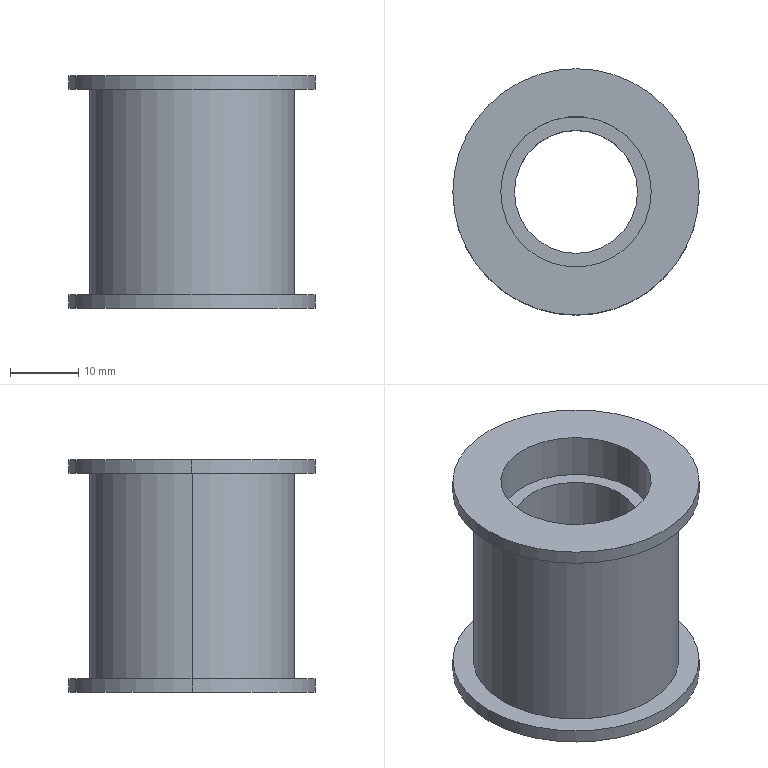Part | STEP file | (PA01.001.LX007) Tensioner Pulley | 1 solid | 18 faces | box 36 x 36 x 34 mm | volume 14967 mm3 | cylinder 12 | plane 6 | commonest cylinder face diameters 22 x4 36 x4 18 x2 30 x2
STEP:
#1=CARTESIAN_POINT('',(0.,0.,0.));
#2=DIRECTION('',(0.,0.,1.));
#3=DIRECTION('',(1.,0.,0.));
#4=AXIS2_PLACEMENT_3D('',#1,#2,#3);
#5=CARTESIAN_POINT('',(-18.,0.,-15.));
#6=VERTEX_POINT('',#5);
#7=CARTESIAN_POINT('',(18.,0.,-15.));
#8=VERTEX_POINT('',#7);
#9=CARTESIAN_POINT('',(0.,0.,-15.));
#10=DIRECTION('',(0.,0.,-1.));
#11=DIRECTION('',(-1.,0.,0.));
#12=AXIS2_PLACEMENT_3D('',#9,#10,#11);
#13=CIRCLE('',#12,18.);
#14=CARTESIAN_POINT('',(0.,0.,-15.));
#15=DIRECTION('',(0.,0.,-1.));
#16=DIRECTION('',(-1.,0.,0.));
#17=AXIS2_PLACEMENT_3D('',#14,#15,#16);
#18=CYLINDRICAL_SURFACE('',#17,18.);
#19=CARTESIAN_POINT('',(0.,0.));
#20=DIRECTION('',(1.,0.));
#21=VECTOR('',#20,1.);
#22=LINE('',#19,#21);
#23=(GEOMETRIC_REPRESENTATION_CONTEXT(2)PARAMETRIC_REPRESENTATION_CONTEXT()REPRESENTATION_CONTEXT('',''));
#24=DEFINITIONAL_REPRESENTATION('',(#22),#23);
#25=PCURVE('',#18,#24);
#26=CARTESIAN_POINT('',(0.,0.,-15.));
#27=DIRECTION('',(0.,0.,-1.));
#28=DIRECTION('',(-1.,0.,0.));
#29=AXIS2_PLACEMENT_3D('',#26,#27,#28);
#30=PLANE('',#29);
#31=CARTESIAN_POINT('',(0.,0.));
#32=DIRECTION('',(1.,0.));
#33=AXIS2_PLACEMENT_2D('',#31,#32);
#34=CIRCLE('',#33,18.);
#35=(GEOMETRIC_REPRESENTATION_CONTEXT(2)PARAMETRIC_REPRESENTATION_CONTEXT()REPRESENTATION_CONTEXT('',''));
#36=DEFINITIONAL_REPRESENTATION('',(#34),#35);
#37=PCURVE('',#30,#36);
#38=SURFACE_CURVE('',#13,(#25,#37),.PCURVE_S1.);
#39=EDGE_CURVE('',#6,#8,#38,.T.);
#40=ORIENTED_EDGE('',*,*,#39,.T.);
#41=CARTESIAN_POINT('',(18.,0.,-17.));
#42=VERTEX_POINT('',#41);
#43=CARTESIAN_POINT('',(18.,0.,-15.));
#44=DIRECTION('',(0.,0.,-1.));
#45=VECTOR('',#44,1.);
#46=LINE('',#43,#45);
#47=CARTESIAN_POINT('',(3.142,0.));
#48=DIRECTION('',(0.,1.));
#49=VECTOR('',#48,1.);
#50=LINE('',#47,#49);
#51=(GEOMETRIC_REPRESENTATION_CONTEXT(2)PARAMETRIC_REPRESENTATION_CONTEXT()REPRESENTATION_CONTEXT('',''));
#52=DEFINITIONAL_REPRESENTATION('',(#50),#51);
#53=PCURVE('',#18,#52);
#54=CARTESIAN_POINT('',(0.,0.,-15.));
#55=DIRECTION('',(0.,0.,-1.));
#56=DIRECTION('',(-1.,0.,0.));
#57=AXIS2_PLACEMENT_3D('',#54,#55,#56);
#58=CYLINDRICAL_SURFACE('',#57,18.);
#59=CARTESIAN_POINT('',(3.142,0.));
#60=DIRECTION('',(0.,1.));
#61=VECTOR('',#60,1.);
#62=LINE('',#59,#61);
#63=(GEOMETRIC_REPRESENTATION_CONTEXT(2)PARAMETRIC_REPRESENTATION_CONTEXT()REPRESENTATION_CONTEXT('',''));
#64=DEFINITIONAL_REPRESENTATION('',(#62),#63);
#65=PCURVE('',#58,#64);
#66=SURFACE_CURVE('',#46,(#53,#65),.PCURVE_S1.);
#67=EDGE_CURVE('',#8,#42,#66,.T.);
#68=ORIENTED_EDGE('',*,*,#67,.T.);
#69=CARTESIAN_POINT('',(-18.,0.,-17.));
#70=VERTEX_POINT('',#69);
#71=CARTESIAN_POINT('',(0.,0.,-17.));
#72=DIRECTION('',(0.,0.,-1.));
#73=DIRECTION('',(-1.,0.,0.));
#74=AXIS2_PLACEMENT_3D('',#71,#72,#73);
#75=CIRCLE('',#74,18.);
#76=CARTESIAN_POINT('',(0.,2.));
#77=DIRECTION('',(1.,0.));
#78=VECTOR('',#77,1.);
#79=LINE('',#76,#78);
#80=(GEOMETRIC_REPRESENTATION_CONTEXT(2)PARAMETRIC_REPRESENTATION_CONTEXT()REPRESENTATION_CONTEXT('',''));
#81=DEFINITIONAL_REPRESENTATION('',(#79),#80);
#82=PCURVE('',#18,#81);
#83=CARTESIAN_POINT('',(0.,0.,-17.));
#84=DIRECTION('',(0.,0.,1.));
#85=DIRECTION('',(1.,0.,0.));
#86=AXIS2_PLACEMENT_3D('',#83,#84,#85);
#87=PLANE('',#86);
#88=CARTESIAN_POINT('',(-18.,0.));
#89=CARTESIAN_POINT('',(-18.,31.177));
#90=CARTESIAN_POINT('',(9.,15.588));
#91=CARTESIAN_POINT('',(36.,0.));
#92=CARTESIAN_POINT('',(9.,-15.588));
#93=CARTESIAN_POINT('',(-18.,-31.177));
#94=CARTESIAN_POINT('',(-18.,0.));
#95=(BOUNDED_CURVE()B_SPLINE_CURVE(2,(#88,#89,#90,#91,#92,#93,#94),.UNSPECIFIED.,.T.,.F.)B_SPLINE_CURVE_WITH_KNOTS((1,2,2,2,2,1),(-2.094,0.,2.094,4.189,6.283,8.378),.UNSPECIFIED.)CURVE()GEOMETRIC_REPRESENTATION_ITEM()RATIONAL_B_SPLINE_CURVE((1.,0.5,1.,0.5,1.,0.5,1.))REPRESENTATION_ITEM(''));
#96=(GEOMETRIC_REPRESENTATION_CONTEXT(2)PARAMETRIC_REPRESENTATION_CONTEXT()REPRESENTATION_CONTEXT('',''));
#97=DEFINITIONAL_REPRESENTATION('',(#95),#96);
#98=PCURVE('',#87,#97);
#99=SURFACE_CURVE('',#75,(#82,#98),.PCURVE_S1.);
#100=EDGE_CURVE('',#70,#42,#99,.T.);
#101=ORIENTED_EDGE('',*,*,#100,.F.);
#102=CARTESIAN_POINT('',(-18.,0.,-15.));
#103=DIRECTION('',(0.,0.,-1.));
#104=VECTOR('',#103,1.);
#105=LINE('',#102,#104);
#106=CARTESIAN_POINT('',(0.,0.));
#107=DIRECTION('',(0.,1.));
#108=VECTOR('',#107,1.);
#109=LINE('',#106,#108);
#110=(GEOMETRIC_REPRESENTATION_CONTEXT(2)PARAMETRIC_REPRESENTATION_CONTEXT()REPRESENTATION_CONTEXT('',''));
#111=DEFINITIONAL_REPRESENTATION('',(#109),#110);
#112=PCURVE('',#18,#111);
#113=CARTESIAN_POINT('',(6.283,0.));
#114=DIRECTION('',(0.,1.));
#115=VECTOR('',#114,1.);
#116=LINE('',#113,#115);
#117=(GEOMETRIC_REPRESENTATION_CONTEXT(2)PARAMETRIC_REPRESENTATION_CONTEXT()REPRESENTATION_CONTEXT('',''));
#118=DEFINITIONAL_REPRESENTATION('',(#116),#117);
#119=PCURVE('',#58,#118);
#120=SURFACE_CURVE('',#105,(#112,#119),.PCURVE_S1.);
#121=EDGE_CURVE('',#6,#70,#120,.T.);
#122=ORIENTED_EDGE('',*,*,#121,.F.);
#123=EDGE_LOOP('',(#40,#68,#101,#122));
#124=FACE_BOUND('',#123,.T.);
#125=ADVANCED_FACE('',(#124),#18,.T.);
#126=CARTESIAN_POINT('',(18.,0.,15.));
#127=VERTEX_POINT('',#126);
#128=CARTESIAN_POINT('',(-18.,0.,15.));
#129=VERTEX_POINT('',#128);
#130=CARTESIAN_POINT('',(0.,0.,15.));
#131=DIRECTION('',(0.,0.,1.));
#132=DIRECTION('',(1.,0.,0.));
#133=AXIS2_PLACEMENT_3D('',#130,#131,#132);
#134=CIRCLE('',#133,18.);
#135=CARTESIAN_POINT('',(0.,0.,15.));
#136=DIRECTION('',(0.,0.,1.));
#137=DIRECTION('',(1.,0.,0.));
#138=AXIS2_PLACEMENT_3D('',#135,#136,#137);
#139=CYLINDRICAL_SURFACE('',#138,18.);
#140=CARTESIAN_POINT('',(0.,0.));
#141=DIRECTION('',(1.,0.));
#142=VECTOR('',#141,1.);
#143=LINE('',#140,#142);
#144=(GEOMETRIC_REPRESENTATION_CONTEXT(2)PARAMETRIC_REPRESENTATION_CONTEXT()REPRESENTATION_CONTEXT('',''));
#145=DEFINITIONAL_REPRESENTATION('',(#143),#144);
#146=PCURVE('',#139,#145);
#147=CARTESIAN_POINT('',(0.,0.,15.));
#148=DIRECTION('',(0.,0.,1.));
#149=DIRECTION('',(1.,0.,0.));
#150=AXIS2_PLACEMENT_3D('',#147,#148,#149);
#151=PLANE('',#150);
#152=CARTESIAN_POINT('',(0.,0.));
#153=DIRECTION('',(1.,0.));
#154=AXIS2_PLACEMENT_2D('',#152,#153);
#155=CIRCLE('',#154,18.);
#156=(GEOMETRIC_REPRESENTATION_CONTEXT(2)PARAMETRIC_REPRESENTATION_CONTEXT()REPRESENTATION_CONTEXT('',''));
#157=DEFINITIONAL_REPRESENTATION('',(#155),#156);
#158=PCURVE('',#151,#157);
#159=SURFACE_CURVE('',#134,(#146,#158),.PCURVE_S1.);
#160=EDGE_CURVE('',#127,#129,#159,.T.);
#161=ORIENTED_EDGE('',*,*,#160,.T.);
#162=CARTESIAN_POINT('',(-18.,0.,17.));
#163=VERTEX_POINT('',#162);
#164=CARTESIAN_POINT('',(-18.,0.,15.));
#165=DIRECTION('',(0.,0.,1.));
#166=VECTOR('',#165,1.);
#167=LINE('',#164,#166);
#168=CARTESIAN_POINT('',(3.142,0.));
#169=DIRECTION('',(0.,1.));
#170=VECTOR('',#169,1.);
#171=LINE('',#168,#170);
#172=(GEOMETRIC_REPRESENTATION_CONTEXT(2)PARAMETRIC_REPRESENTATION_CONTEXT()REPRESENTATION_CONTEXT('',''));
#173=DEFINITIONAL_REPRESENTATION('',(#171),#172);
#174=PCURVE('',#139,#173);
#175=CARTESIAN_POINT('',(0.,0.,15.));
#176=DIRECTION('',(0.,0.,1.));
#177=DIRECTION('',(1.,0.,0.));
#178=AXIS2_PLACEMENT_3D('',#175,#176,#177);
#179=CYLINDRICAL_SURFACE('',#178,18.);
#180=CARTESIAN_POINT('',(3.142,0.));
#181=DIRECTION('',(0.,1.));
#182=VECTOR('',#181,1.);
#183=LINE('',#180,#182);
#184=(GEOMETRIC_REPRESENTATION_CONTEXT(2)PARAMETRIC_REPRESENTATION_CONTEXT()REPRESENTATION_CONTEXT('',''));
#185=DEFINITIONAL_REPRESENTATION('',(#183),#184);
#186=PCURVE('',#179,#185);
#187=SURFACE_CURVE('',#167,(#174,#186),.PCURVE_S1.);
#188=EDGE_CURVE('',#129,#163,#187,.T.);
#189=ORIENTED_EDGE('',*,*,#188,.T.);
#190=CARTESIAN_POINT('',(18.,0.,17.));
#191=VERTEX_POINT('',#190);
#192=CARTESIAN_POINT('',(0.,0.,17.));
#193=DIRECTION('',(0.,0.,1.));
#194=DIRECTION('',(1.,0.,0.));
#195=AXIS2_PLACEMENT_3D('',#192,#193,#194);
#196=CIRCLE('',#195,18.);
#197=CARTESIAN_POINT('',(0.,2.));
#198=DIRECTION('',(1.,0.));
#199=VECTOR('',#198,1.);
#200=LINE('',#197,#199);
#201=(GEOMETRIC_REPRESENTATION_CONTEXT(2)PARAMETRIC_REPRESENTATION_CONTEXT()REPRESENTATION_CONTEXT('',''));
#202=DEFINITIONAL_REPRESENTATION('',(#200),#201);
#203=PCURVE('',#139,#202);
#204=CARTESIAN_POINT('',(0.,0.,17.));
#205=DIRECTION('',(0.,0.,1.));
#206=DIRECTION('',(1.,0.,0.));
#207=AXIS2_PLACEMENT_3D('',#204,#205,#206);
#208=PLANE('',#207);
#209=CARTESIAN_POINT('',(0.,0.));
#210=DIRECTION('',(1.,0.));
#211=AXIS2_PLACEMENT_2D('',#209,#210);
#212=CIRCLE('',#211,18.);
#213=(GEOMETRIC_REPRESENTATION_CONTEXT(2)PARAMETRIC_REPRESENTATION_CONTEXT()REPRESENTATION_CONTEXT('',''));
#214=DEFINITIONAL_REPRESENTATION('',(#212),#213);
#215=PCURVE('',#208,#214);
#216=SURFACE_CURVE('',#196,(#203,#215),.PCURVE_S1.);
#217=EDGE_CURVE('',#191,#163,#216,.T.);
#218=ORIENTED_EDGE('',*,*,#217,.F.);
#219=CARTESIAN_POINT('',(18.,0.,15.));
#220=DIRECTION('',(0.,0.,1.));
#221=VECTOR('',#220,1.);
#222=LINE('',#219,#221);
#223=CARTESIAN_POINT('',(0.,0.));
#224=DIRECTION('',(0.,1.));
#225=VECTOR('',#224,1.);
#226=LINE('',#223,#225);
#227=(GEOMETRIC_REPRESENTATION_CONTEXT(2)PARAMETRIC_REPRESENTATION_CONTEXT()REPRESENTATION_CONTEXT('',''));
#228=DEFINITIONAL_REPRESENTATION('',(#226),#227);
#229=PCURVE('',#139,#228);
#230=CARTESIAN_POINT('',(6.283,0.));
#231=DIRECTION('',(0.,1.));
#232=VECTOR('',#231,1.);
#233=LINE('',#230,#232);
#234=(GEOMETRIC_REPRESENTATION_CONTEXT(2)PARAMETRIC_REPRESENTATION_CONTEXT()REPRESENTATION_CONTEXT('',''));
#235=DEFINITIONAL_REPRESENTATION('',(#233),#234);
#236=PCURVE('',#179,#235);
#237=SURFACE_CURVE('',#222,(#229,#236),.PCURVE_S1.);
#238=EDGE_CURVE('',#127,#191,#237,.T.);
#239=ORIENTED_EDGE('',*,*,#238,.F.);
#240=EDGE_LOOP('',(#161,#189,#218,#239));
#241=FACE_BOUND('',#240,.T.);
#242=ADVANCED_FACE('',(#241),#139,.T.);
#243=CARTESIAN_POINT('',(9.,0.,-10.4));
#244=VERTEX_POINT('',#243);
#245=CARTESIAN_POINT('',(9.,0.,10.4));
#246=VERTEX_POINT('',#245);
#247=CARTESIAN_POINT('',(9.,0.,-17.));
#248=DIRECTION('',(0.,0.,1.));
#249=VECTOR('',#248,1.);
#250=LINE('',#247,#249);
#251=CARTESIAN_POINT('',(0.,0.,-17.));
#252=DIRECTION('',(0.,0.,1.));
#253=DIRECTION('',(1.,0.,0.));
#254=AXIS2_PLACEMENT_3D('',#251,#252,#253);
#255=CYLINDRICAL_SURFACE('',#254,9.);
#256=CARTESIAN_POINT('',(6.283,0.));
#257=DIRECTION('',(0.,1.));
#258=VECTOR('',#257,1.);
#259=LINE('',#256,#258);
#260=(GEOMETRIC_REPRESENTATION_CONTEXT(2)PARAMETRIC_REPRESENTATION_CONTEXT()REPRESENTATION_CONTEXT('',''));
#261=DEFINITIONAL_REPRESENTATION('',(#259),#260);
#262=PCURVE('',#255,#261);
#263=CARTESIAN_POINT('',(0.,0.,-17.));
#264=DIRECTION('',(0.,0.,1.));
#265=DIRECTION('',(1.,0.,0.));
#266=AXIS2_PLACEMENT_3D('',#263,#264,#265);
#267=CYLINDRICAL_SURFACE('',#266,9.);
#268=CARTESIAN_POINT('',(0.,0.));
#269=DIRECTION('',(0.,1.));
#270=VECTOR('',#269,1.);
#271=LINE('',#268,#270);
#272=(GEOMETRIC_REPRESENTATION_CONTEXT(2)PARAMETRIC_REPRESENTATION_CONTEXT()REPRESENTATION_CONTEXT('',''));
#273=DEFINITIONAL_REPRESENTATION('',(#271),#272);
#274=PCURVE('',#267,#273);
#275=SURFACE_CURVE('',#250,(#262,#274),.PCURVE_S1.);
#276=EDGE_CURVE('',#244,#246,#275,.T.);
#277=ORIENTED_EDGE('',*,*,#276,.T.);
#278=CARTESIAN_POINT('',(-9.,0.,10.4));
#279=VERTEX_POINT('',#278);
#280=CARTESIAN_POINT('',(0.,0.,10.4));
#281=DIRECTION('',(0.,0.,1.));
#282=DIRECTION('',(1.,0.,0.));
#283=AXIS2_PLACEMENT_3D('',#280,#281,#282);
#284=CIRCLE('',#283,9.);
#285=CARTESIAN_POINT('',(0.,27.4));
#286=DIRECTION('',(1.,0.));
#287=VECTOR('',#286,1.);
#288=LINE('',#285,#287);
#289=(GEOMETRIC_REPRESENTATION_CONTEXT(2)PARAMETRIC_REPRESENTATION_CONTEXT()REPRESENTATION_CONTEXT('',''));
#290=DEFINITIONAL_REPRESENTATION('',(#288),#289);
#291=PCURVE('',#255,#290);
#292=CARTESIAN_POINT('',(0.,0.,10.4));
#293=DIRECTION('',(0.,0.,1.));
#294=DIRECTION('',(1.,0.,0.));
#295=AXIS2_PLACEMENT_3D('',#292,#293,#294);
#296=PLANE('',#295);
#297=CARTESIAN_POINT('',(0.,0.));
#298=DIRECTION('',(1.,0.));
#299=AXIS2_PLACEMENT_2D('',#297,#298);
#300=CIRCLE('',#299,9.);
#301=(GEOMETRIC_REPRESENTATION_CONTEXT(2)PARAMETRIC_REPRESENTATION_CONTEXT()REPRESENTATION_CONTEXT('',''));
#302=DEFINITIONAL_REPRESENTATION('',(#300),#301);
#303=PCURVE('',#296,#302);
#304=SURFACE_CURVE('',#284,(#291,#303),.PCURVE_S1.);
#305=EDGE_CURVE('',#279,#246,#304,.T.);
#306=ORIENTED_EDGE('',*,*,#305,.F.);
#307=CARTESIAN_POINT('',(-9.,0.,-10.4));
#308=VERTEX_POINT('',#307);
#309=CARTESIAN_POINT('',(-9.,0.,-17.));
#310=DIRECTION('',(0.,0.,1.));
#311=VECTOR('',#310,1.);
#312=LINE('',#309,#311);
#313=CARTESIAN_POINT('',(3.142,0.));
#314=DIRECTION('',(0.,1.));
#315=VECTOR('',#314,1.);
#316=LINE('',#313,#315);
#317=(GEOMETRIC_REPRESENTATION_CONTEXT(2)PARAMETRIC_REPRESENTATION_CONTEXT()REPRESENTATION_CONTEXT('',''));
#318=DEFINITIONAL_REPRESENTATION('',(#316),#317);
#319=PCURVE('',#255,#318);
#320=CARTESIAN_POINT('',(3.142,0.));
#321=DIRECTION('',(0.,1.));
#322=VECTOR('',#321,1.);
#323=LINE('',#320,#322);
#324=(GEOMETRIC_REPRESENTATION_CONTEXT(2)PARAMETRIC_REPRESENTATION_CONTEXT()REPRESENTATION_CONTEXT('',''));
#325=DEFINITIONAL_REPRESENTATION('',(#323),#324);
#326=PCURVE('',#267,#325);
#327=SURFACE_CURVE('',#312,(#319,#326),.PCURVE_S1.);
#328=EDGE_CURVE('',#308,#279,#327,.T.);
#329=ORIENTED_EDGE('',*,*,#328,.F.);
#330=CARTESIAN_POINT('',(0.,0.,-10.4));
#331=DIRECTION('',(0.,0.,-1.));
#332=DIRECTION('',(-1.,0.,0.));
#333=AXIS2_PLACEMENT_3D('',#330,#331,#332);
#334=CIRCLE('',#333,9.);
#335=CARTESIAN_POINT('',(9.425,6.6));
#336=DIRECTION('',(-1.,0.));
#337=VECTOR('',#336,1.);
#338=LINE('',#335,#337);
#339=(GEOMETRIC_REPRESENTATION_CONTEXT(2)PARAMETRIC_REPRESENTATION_CONTEXT()REPRESENTATION_CONTEXT('',''));
#340=DEFINITIONAL_REPRESENTATION('',(#338),#339);
#341=PCURVE('',#255,#340);
#342=CARTESIAN_POINT('',(0.,0.,-10.4));
#343=DIRECTION('',(0.,0.,-1.));
#344=DIRECTION('',(1.,0.,0.));
#345=AXIS2_PLACEMENT_3D('',#342,#343,#344);
#346=PLANE('',#345);
#347=CARTESIAN_POINT('',(0.,0.));
#348=DIRECTION('',(-1.,0.));
#349=AXIS2_PLACEMENT_2D('',#347,#348);
#350=CIRCLE('',#349,9.);
#351=(GEOMETRIC_REPRESENTATION_CONTEXT(2)PARAMETRIC_REPRESENTATION_CONTEXT()REPRESENTATION_CONTEXT('',''));
#352=DEFINITIONAL_REPRESENTATION('',(#350),#351);
#353=PCURVE('',#346,#352);
#354=SURFACE_CURVE('',#334,(#341,#353),.PCURVE_S1.);
#355=EDGE_CURVE('',#244,#308,#354,.T.);
#356=ORIENTED_EDGE('',*,*,#355,.F.);
#357=EDGE_LOOP('',(#277,#306,#329,#356));
#358=FACE_BOUND('',#357,.F.);
#359=ADVANCED_FACE('',(#358),#255,.F.);
#360=CARTESIAN_POINT('',(-11.,0.,-10.4));
#361=VERTEX_POINT('',#360);
#362=CARTESIAN_POINT('',(-11.,0.,-17.));
#363=VERTEX_POINT('',#362);
#364=CARTESIAN_POINT('',(-11.,0.,-10.4));
#365=DIRECTION('',(0.,0.,-1.));
#366=VECTOR('',#365,1.);
#367=LINE('',#364,#366);
#368=CARTESIAN_POINT('',(0.,0.,-10.4));
#369=DIRECTION('',(0.,0.,-1.));
#370=DIRECTION('',(-1.,0.,0.));
#371=AXIS2_PLACEMENT_3D('',#368,#369,#370);
#372=CYLINDRICAL_SURFACE('',#371,11.);
#373=CARTESIAN_POINT('',(6.283,0.));
#374=DIRECTION('',(0.,1.));
#375=VECTOR('',#374,1.);
#376=LINE('',#373,#375);
#377=(GEOMETRIC_REPRESENTATION_CONTEXT(2)PARAMETRIC_REPRESENTATION_CONTEXT()REPRESENTATION_CONTEXT('',''));
#378=DEFINITIONAL_REPRESENTATION('',(#376),#377);
#379=PCURVE('',#372,#378);
#380=CARTESIAN_POINT('',(0.,0.,-10.4));
#381=DIRECTION('',(0.,0.,-1.));
#382=DIRECTION('',(-1.,0.,0.));
#383=AXIS2_PLACEMENT_3D('',#380,#381,#382);
#384=CYLINDRICAL_SURFACE('',#383,11.);
#385=CARTESIAN_POINT('',(0.,0.));
#386=DIRECTION('',(0.,1.));
#387=VECTOR('',#386,1.);
#388=LINE('',#385,#387);
#389=(GEOMETRIC_REPRESENTATION_CONTEXT(2)PARAMETRIC_REPRESENTATION_CONTEXT()REPRESENTATION_CONTEXT('',''));
#390=DEFINITIONAL_REPRESENTATION('',(#388),#389);
#391=PCURVE('',#384,#390);
#392=SURFACE_CURVE('',#367,(#379,#391),.PCURVE_S1.);
#393=EDGE_CURVE('',#361,#363,#392,.T.);
#394=ORIENTED_EDGE('',*,*,#393,.T.);
#395=CARTESIAN_POINT('',(11.,0.,-17.));
#396=VERTEX_POINT('',#395);
#397=CARTESIAN_POINT('',(0.,0.,-17.));
#398=DIRECTION('',(0.,0.,1.));
#399=DIRECTION('',(1.,0.,0.));
#400=AXIS2_PLACEMENT_3D('',#397,#398,#399);
#401=CIRCLE('',#400,11.);
#402=CARTESIAN_POINT('',(9.425,6.6));
#403=DIRECTION('',(-1.,0.));
#404=VECTOR('',#403,1.);
#405=LINE('',#402,#404);
#406=(GEOMETRIC_REPRESENTATION_CONTEXT(2)PARAMETRIC_REPRESENTATION_CONTEXT()REPRESENTATION_CONTEXT('',''));
#407=DEFINITIONAL_REPRESENTATION('',(#405),#406);
#408=PCURVE('',#372,#407);
#409=CARTESIAN_POINT('',(0.,0.));
#410=DIRECTION('',(1.,0.));
#411=AXIS2_PLACEMENT_2D('',#409,#410);
#412=CIRCLE('',#411,11.);
#413=(GEOMETRIC_REPRESENTATION_CONTEXT(2)PARAMETRIC_REPRESENTATION_CONTEXT()REPRESENTATION_CONTEXT('',''));
#414=DEFINITIONAL_REPRESENTATION('',(#412),#413);
#415=PCURVE('',#87,#414);
#416=SURFACE_CURVE('',#401,(#408,#415),.PCURVE_S1.);
#417=EDGE_CURVE('',#363,#396,#416,.T.);
#418=ORIENTED_EDGE('',*,*,#417,.T.);
#419=CARTESIAN_POINT('',(11.,0.,-10.4));
#420=VERTEX_POINT('',#419);
#421=CARTESIAN_POINT('',(11.,0.,-10.4));
#422=DIRECTION('',(0.,0.,-1.));
#423=VECTOR('',#422,1.);
#424=LINE('',#421,#423);
#425=CARTESIAN_POINT('',(3.142,0.));
#426=DIRECTION('',(0.,1.));
#427=VECTOR('',#426,1.);
#428=LINE('',#425,#427);
#429=(GEOMETRIC_REPRESENTATION_CONTEXT(2)PARAMETRIC_REPRESENTATION_CONTEXT()REPRESENTATION_CONTEXT('',''));
#430=DEFINITIONAL_REPRESENTATION('',(#428),#429);
#431=PCURVE('',#372,#430);
#432=CARTESIAN_POINT('',(3.142,0.));
#433=DIRECTION('',(0.,1.));
#434=VECTOR('',#433,1.);
#435=LINE('',#432,#434);
#436=(GEOMETRIC_REPRESENTATION_CONTEXT(2)PARAMETRIC_REPRESENTATION_CONTEXT()REPRESENTATION_CONTEXT('',''));
#437=DEFINITIONAL_REPRESENTATION('',(#435),#436);
#438=PCURVE('',#384,#437);
#439=SURFACE_CURVE('',#424,(#431,#438),.PCURVE_S1.);
#440=EDGE_CURVE('',#420,#396,#439,.T.);
#441=ORIENTED_EDGE('',*,*,#440,.F.);
#442=CARTESIAN_POINT('',(0.,0.,-10.4));
#443=DIRECTION('',(0.,0.,1.));
#444=DIRECTION('',(1.,0.,0.));
#445=AXIS2_PLACEMENT_3D('',#442,#443,#444);
#446=CIRCLE('',#445,11.);
#447=CARTESIAN_POINT('',(9.425,0.));
#448=DIRECTION('',(-1.,0.));
#449=VECTOR('',#448,1.);
#450=LINE('',#447,#449);
#451=(GEOMETRIC_REPRESENTATION_CONTEXT(2)PARAMETRIC_REPRESENTATION_CONTEXT()REPRESENTATION_CONTEXT('',''));
#452=DEFINITIONAL_REPRESENTATION('',(#450),#451);
#453=PCURVE('',#372,#452);
#454=CARTESIAN_POINT('',(11.,0.));
#455=CARTESIAN_POINT('',(11.,-19.053));
#456=CARTESIAN_POINT('',(-5.5,-9.526));
#457=CARTESIAN_POINT('',(-22.,0.));
#458=CARTESIAN_POINT('',(-5.5,9.526));
#459=CARTESIAN_POINT('',(11.,19.053));
#460=CARTESIAN_POINT('',(11.,0.));
#461=(BOUNDED_CURVE()B_SPLINE_CURVE(2,(#454,#455,#456,#457,#458,#459,#460),.UNSPECIFIED.,.T.,.F.)B_SPLINE_CURVE_WITH_KNOTS((1,2,2,2,2,1),(-2.094,0.,2.094,4.189,6.283,8.378),.UNSPECIFIED.)CURVE()GEOMETRIC_REPRESENTATION_ITEM()RATIONAL_B_SPLINE_CURVE((1.,0.5,1.,0.5,1.,0.5,1.))REPRESENTATION_ITEM(''));
#462=(GEOMETRIC_REPRESENTATION_CONTEXT(2)PARAMETRIC_REPRESENTATION_CONTEXT()REPRESENTATION_CONTEXT('',''));
#463=DEFINITIONAL_REPRESENTATION('',(#461),#462);
#464=PCURVE('',#346,#463);
#465=SURFACE_CURVE('',#446,(#453,#464),.PCURVE_S1.);
#466=EDGE_CURVE('',#361,#420,#465,.T.);
#467=ORIENTED_EDGE('',*,*,#466,.F.);
#468=EDGE_LOOP('',(#394,#418,#441,#467));
#469=FACE_BOUND('',#468,.F.);
#470=ADVANCED_FACE('',(#469),#372,.F.);
#471=CARTESIAN_POINT('',(11.,0.,10.4));
#472=VERTEX_POINT('',#471);
#473=CARTESIAN_POINT('',(11.,0.,17.));
#474=VERTEX_POINT('',#473);
#475=CARTESIAN_POINT('',(11.,0.,10.4));
#476=DIRECTION('',(0.,0.,1.));
#477=VECTOR('',#476,1.);
#478=LINE('',#475,#477);
#479=CARTESIAN_POINT('',(0.,0.,10.4));
#480=DIRECTION('',(0.,0.,1.));
#481=DIRECTION('',(1.,0.,0.));
#482=AXIS2_PLACEMENT_3D('',#479,#480,#481);
#483=CYLINDRICAL_SURFACE('',#482,11.);
#484=CARTESIAN_POINT('',(6.283,0.));
#485=DIRECTION('',(0.,1.));
#486=VECTOR('',#485,1.);
#487=LINE('',#484,#486);
#488=(GEOMETRIC_REPRESENTATION_CONTEXT(2)PARAMETRIC_REPRESENTATION_CONTEXT()REPRESENTATION_CONTEXT('',''));
#489=DEFINITIONAL_REPRESENTATION('',(#487),#488);
#490=PCURVE('',#483,#489);
#491=CARTESIAN_POINT('',(0.,0.,10.4));
#492=DIRECTION('',(0.,0.,1.));
#493=DIRECTION('',(1.,0.,0.));
#494=AXIS2_PLACEMENT_3D('',#491,#492,#493);
#495=CYLINDRICAL_SURFACE('',#494,11.);
#496=CARTESIAN_POINT('',(0.,0.));
#497=DIRECTION('',(0.,1.));
#498=VECTOR('',#497,1.);
#499=LINE('',#496,#498);
#500=(GEOMETRIC_REPRESENTATION_CONTEXT(2)PARAMETRIC_REPRESENTATION_CONTEXT()REPRESENTATION_CONTEXT('',''));
#501=DEFINITIONAL_REPRESENTATION('',(#499),#500);
#502=PCURVE('',#495,#501);
#503=SURFACE_CURVE('',#478,(#490,#502),.PCURVE_S1.);
#504=EDGE_CURVE('',#472,#474,#503,.T.);
#505=ORIENTED_EDGE('',*,*,#504,.T.);
#506=CARTESIAN_POINT('',(-11.,0.,17.));
#507=VERTEX_POINT('',#506);
#508=CARTESIAN_POINT('',(0.,0.,17.));
#509=DIRECTION('',(0.,0.,1.));
#510=DIRECTION('',(1.,0.,0.));
#511=AXIS2_PLACEMENT_3D('',#508,#509,#510);
#512=CIRCLE('',#511,11.);
#513=CARTESIAN_POINT('',(0.,6.6));
#514=DIRECTION('',(1.,0.));
#515=VECTOR('',#514,1.);
#516=LINE('',#513,#515);
#517=(GEOMETRIC_REPRESENTATION_CONTEXT(2)PARAMETRIC_REPRESENTATION_CONTEXT()REPRESENTATION_CONTEXT('',''));
#518=DEFINITIONAL_REPRESENTATION('',(#516),#517);
#519=PCURVE('',#483,#518);
#520=CARTESIAN_POINT('',(0.,0.));
#521=DIRECTION('',(1.,0.));
#522=AXIS2_PLACEMENT_2D('',#520,#521);
#523=CIRCLE('',#522,11.);
#524=(GEOMETRIC_REPRESENTATION_CONTEXT(2)PARAMETRIC_REPRESENTATION_CONTEXT()REPRESENTATION_CONTEXT('',''));
#525=DEFINITIONAL_REPRESENTATION('',(#523),#524);
#526=PCURVE('',#208,#525);
#527=SURFACE_CURVE('',#512,(#519,#526),.PCURVE_S1.);
#528=EDGE_CURVE('',#507,#474,#527,.T.);
#529=ORIENTED_EDGE('',*,*,#528,.F.);
#530=CARTESIAN_POINT('',(-11.,0.,10.4));
#531=VERTEX_POINT('',#530);
#532=CARTESIAN_POINT('',(-11.,0.,10.4));
#533=DIRECTION('',(0.,0.,1.));
#534=VECTOR('',#533,1.);
#535=LINE('',#532,#534);
#536=CARTESIAN_POINT('',(3.142,0.));
#537=DIRECTION('',(0.,1.));
#538=VECTOR('',#537,1.);
#539=LINE('',#536,#538);
#540=(GEOMETRIC_REPRESENTATION_CONTEXT(2)PARAMETRIC_REPRESENTATION_CONTEXT()REPRESENTATION_CONTEXT('',''));
#541=DEFINITIONAL_REPRESENTATION('',(#539),#540);
#542=PCURVE('',#483,#541);
#543=CARTESIAN_POINT('',(3.142,0.));
#544=DIRECTION('',(0.,1.));
#545=VECTOR('',#544,1.);
#546=LINE('',#543,#545);
#547=(GEOMETRIC_REPRESENTATION_CONTEXT(2)PARAMETRIC_REPRESENTATION_CONTEXT()REPRESENTATION_CONTEXT('',''));
#548=DEFINITIONAL_REPRESENTATION('',(#546),#547);
#549=PCURVE('',#495,#548);
#550=SURFACE_CURVE('',#535,(#542,#549),.PCURVE_S1.);
#551=EDGE_CURVE('',#531,#507,#550,.T.);
#552=ORIENTED_EDGE('',*,*,#551,.F.);
#553=CARTESIAN_POINT('',(0.,0.,10.4));
#554=DIRECTION('',(0.,0.,1.));
#555=DIRECTION('',(1.,0.,0.));
#556=AXIS2_PLACEMENT_3D('',#553,#554,#555);
#557=CIRCLE('',#556,11.);
#558=CARTESIAN_POINT('',(0.,0.));
#559=DIRECTION('',(1.,0.));
#560=VECTOR('',#559,1.);
#561=LINE('',#558,#560);
#562=(GEOMETRIC_REPRESENTATION_CONTEXT(2)PARAMETRIC_REPRESENTATION_CONTEXT()REPRESENTATION_CONTEXT('',''));
#563=DEFINITIONAL_REPRESENTATION('',(#561),#562);
#564=PCURVE('',#483,#563);
#565=CARTESIAN_POINT('',(0.,0.));
#566=DIRECTION('',(1.,0.));
#567=AXIS2_PLACEMENT_2D('',#565,#566);
#568=CIRCLE('',#567,11.);
#569=(GEOMETRIC_REPRESENTATION_CONTEXT(2)PARAMETRIC_REPRESENTATION_CONTEXT()REPRESENTATION_CONTEXT('',''));
#570=DEFINITIONAL_REPRESENTATION('',(#568),#569);
#571=PCURVE('',#296,#570);
#572=SURFACE_CURVE('',#557,(#564,#571),.PCURVE_S1.);
#573=EDGE_CURVE('',#531,#472,#572,.T.);
#574=ORIENTED_EDGE('',*,*,#573,.T.);
#575=EDGE_LOOP('',(#505,#529,#552,#574));
#576=FACE_BOUND('',#575,.F.);
#577=ADVANCED_FACE('',(#576),#483,.F.);
#578=CARTESIAN_POINT('',(15.,0.,15.));
#579=VERTEX_POINT('',#578);
#580=CARTESIAN_POINT('',(-15.,0.,15.));
#581=VERTEX_POINT('',#580);
#582=CARTESIAN_POINT('',(0.,0.,15.));
#583=DIRECTION('',(0.,0.,1.));
#584=DIRECTION('',(1.,0.,0.));
#585=AXIS2_PLACEMENT_3D('',#582,#583,#584);
#586=CIRCLE('',#585,15.);
#587=CARTESIAN_POINT('',(0.,0.,17.));
#588=DIRECTION('',(0.,0.,-1.));
#589=DIRECTION('',(-1.,0.,0.));
#590=AXIS2_PLACEMENT_3D('',#587,#588,#589);
#591=CYLINDRICAL_SURFACE('',#590,15.);
#592=CARTESIAN_POINT('',(3.142,2.));
#593=DIRECTION('',(-1.,0.));
#594=VECTOR('',#593,1.);
#595=LINE('',#592,#594);
#596=(GEOMETRIC_REPRESENTATION_CONTEXT(2)PARAMETRIC_REPRESENTATION_CONTEXT()REPRESENTATION_CONTEXT('',''));
#597=DEFINITIONAL_REPRESENTATION('',(#595),#596);
#598=PCURVE('',#591,#597);
#599=CARTESIAN_POINT('',(0.,0.));
#600=DIRECTION('',(1.,0.));
#601=AXIS2_PLACEMENT_2D('',#599,#600);
#602=CIRCLE('',#601,15.);
#603=(GEOMETRIC_REPRESENTATION_CONTEXT(2)PARAMETRIC_REPRESENTATION_CONTEXT()REPRESENTATION_CONTEXT('',''));
#604=DEFINITIONAL_REPRESENTATION('',(#602),#603);
#605=PCURVE('',#151,#604);
#606=SURFACE_CURVE('',#586,(#598,#605),.PCURVE_S1.);
#607=EDGE_CURVE('',#579,#581,#606,.T.);
#608=ORIENTED_EDGE('',*,*,#607,.F.);
#609=CARTESIAN_POINT('',(15.,0.,-15.));
#610=VERTEX_POINT('',#609);
#611=CARTESIAN_POINT('',(15.,0.,17.));
#612=DIRECTION('',(0.,0.,-1.));
#613=VECTOR('',#612,1.);
#614=LINE('',#611,#613);
#615=CARTESIAN_POINT('',(3.142,0.));
#616=DIRECTION('',(0.,1.));
#617=VECTOR('',#616,1.);
#618=LINE('',#615,#617);
#619=(GEOMETRIC_REPRESENTATION_CONTEXT(2)PARAMETRIC_REPRESENTATION_CONTEXT()REPRESENTATION_CONTEXT('',''));
#620=DEFINITIONAL_REPRESENTATION('',(#618),#619);
#621=PCURVE('',#591,#620);
#622=CARTESIAN_POINT('',(0.,0.,17.));
#623=DIRECTION('',(0.,0.,-1.));
#624=DIRECTION('',(-1.,0.,0.));
#625=AXIS2_PLACEMENT_3D('',#622,#623,#624);
#626=CYLINDRICAL_SURFACE('',#625,15.);
#627=CARTESIAN_POINT('',(3.142,0.));
#628=DIRECTION('',(0.,1.));
#629=VECTOR('',#628,1.);
#630=LINE('',#627,#629);
#631=(GEOMETRIC_REPRESENTATION_CONTEXT(2)PARAMETRIC_REPRESENTATION_CONTEXT()REPRESENTATION_CONTEXT('',''));
#632=DEFINITIONAL_REPRESENTATION('',(#630),#631);
#633=PCURVE('',#626,#632);
#634=SURFACE_CURVE('',#614,(#621,#633),.PCURVE_S1.);
#635=EDGE_CURVE('',#579,#610,#634,.T.);
#636=ORIENTED_EDGE('',*,*,#635,.T.);
#637=CARTESIAN_POINT('',(-15.,0.,-15.));
#638=VERTEX_POINT('',#637);
#639=CARTESIAN_POINT('',(0.,0.,-15.));
#640=DIRECTION('',(0.,0.,-1.));
#641=DIRECTION('',(-1.,0.,0.));
#642=AXIS2_PLACEMENT_3D('',#639,#640,#641);
#643=CIRCLE('',#642,15.);
#644=CARTESIAN_POINT('',(0.,32.));
#645=DIRECTION('',(1.,0.));
#646=VECTOR('',#645,1.);
#647=LINE('',#644,#646);
#648=(GEOMETRIC_REPRESENTATION_CONTEXT(2)PARAMETRIC_REPRESENTATION_CONTEXT()REPRESENTATION_CONTEXT('',''));
#649=DEFINITIONAL_REPRESENTATION('',(#647),#648);
#650=PCURVE('',#591,#649);
#651=CARTESIAN_POINT('',(0.,0.));
#652=DIRECTION('',(1.,0.));
#653=AXIS2_PLACEMENT_2D('',#651,#652);
#654=CIRCLE('',#653,15.);
#655=(GEOMETRIC_REPRESENTATION_CONTEXT(2)PARAMETRIC_REPRESENTATION_CONTEXT()REPRESENTATION_CONTEXT('',''));
#656=DEFINITIONAL_REPRESENTATION('',(#654),#655);
#657=PCURVE('',#30,#656);
#658=SURFACE_CURVE('',#643,(#650,#657),.PCURVE_S1.);
#659=EDGE_CURVE('',#638,#610,#658,.T.);
#660=ORIENTED_EDGE('',*,*,#659,.F.);
#661=CARTESIAN_POINT('',(-15.,0.,17.));
#662=DIRECTION('',(0.,0.,-1.));
#663=VECTOR('',#662,1.);
#664=LINE('',#661,#663);
#665=CARTESIAN_POINT('',(0.,0.));
#666=DIRECTION('',(0.,1.));
#667=VECTOR('',#666,1.);
#668=LINE('',#665,#667);
#669=(GEOMETRIC_REPRESENTATION_CONTEXT(2)PARAMETRIC_REPRESENTATION_CONTEXT()REPRESENTATION_CONTEXT('',''));
#670=DEFINITIONAL_REPRESENTATION('',(#668),#669);
#671=PCURVE('',#591,#670);
#672=CARTESIAN_POINT('',(6.283,0.));
#673=DIRECTION('',(0.,1.));
#674=VECTOR('',#673,1.);
#675=LINE('',#672,#674);
#676=(GEOMETRIC_REPRESENTATION_CONTEXT(2)PARAMETRIC_REPRESENTATION_CONTEXT()REPRESENTATION_CONTEXT('',''));
#677=DEFINITIONAL_REPRESENTATION('',(#675),#676);
#678=PCURVE('',#626,#677);
#679=SURFACE_CURVE('',#664,(#671,#678),.PCURVE_S1.);
#680=EDGE_CURVE('',#581,#638,#679,.T.);
#681=ORIENTED_EDGE('',*,*,#680,.F.);
#682=EDGE_LOOP('',(#608,#636,#660,#681));
#683=FACE_BOUND('',#682,.T.);
#684=ADVANCED_FACE('',(#683),#591,.T.);
#685=ORIENTED_EDGE('',*,*,#635,.F.);
#686=CARTESIAN_POINT('',(0.,0.,15.));
#687=DIRECTION('',(0.,0.,1.));
#688=DIRECTION('',(1.,0.,0.));
#689=AXIS2_PLACEMENT_3D('',#686,#687,#688);
#690=CIRCLE('',#689,15.);
#691=CARTESIAN_POINT('',(9.425,2.));
#692=DIRECTION('',(-1.,0.));
#693=VECTOR('',#692,1.);
#694=LINE('',#691,#693);
#695=(GEOMETRIC_REPRESENTATION_CONTEXT(2)PARAMETRIC_REPRESENTATION_CONTEXT()REPRESENTATION_CONTEXT('',''));
#696=DEFINITIONAL_REPRESENTATION('',(#694),#695);
#697=PCURVE('',#626,#696);
#698=CARTESIAN_POINT('',(0.,0.));
#699=DIRECTION('',(1.,0.));
#700=AXIS2_PLACEMENT_2D('',#698,#699);
#701=CIRCLE('',#700,15.);
#702=(GEOMETRIC_REPRESENTATION_CONTEXT(2)PARAMETRIC_REPRESENTATION_CONTEXT()REPRESENTATION_CONTEXT('',''));
#703=DEFINITIONAL_REPRESENTATION('',(#701),#702);
#704=PCURVE('',#151,#703);
#705=SURFACE_CURVE('',#690,(#697,#704),.PCURVE_S1.);
#706=EDGE_CURVE('',#581,#579,#705,.T.);
#707=ORIENTED_EDGE('',*,*,#706,.F.);
#708=ORIENTED_EDGE('',*,*,#680,.T.);
#709=CARTESIAN_POINT('',(0.,0.,-15.));
#710=DIRECTION('',(0.,0.,-1.));
#711=DIRECTION('',(-1.,0.,0.));
#712=AXIS2_PLACEMENT_3D('',#709,#710,#711);
#713=CIRCLE('',#712,15.);
#714=CARTESIAN_POINT('',(0.,32.));
#715=DIRECTION('',(1.,0.));
#716=VECTOR('',#715,1.);
#717=LINE('',#714,#716);
#718=(GEOMETRIC_REPRESENTATION_CONTEXT(2)PARAMETRIC_REPRESENTATION_CONTEXT()REPRESENTATION_CONTEXT('',''));
#719=DEFINITIONAL_REPRESENTATION('',(#717),#718);
#720=PCURVE('',#626,#719);
#721=CARTESIAN_POINT('',(0.,0.));
#722=DIRECTION('',(1.,0.));
#723=AXIS2_PLACEMENT_2D('',#721,#722);
#724=CIRCLE('',#723,15.);
#725=(GEOMETRIC_REPRESENTATION_CONTEXT(2)PARAMETRIC_REPRESENTATION_CONTEXT()REPRESENTATION_CONTEXT('',''));
#726=DEFINITIONAL_REPRESENTATION('',(#724),#725);
#727=PCURVE('',#30,#726);
#728=SURFACE_CURVE('',#713,(#720,#727),.PCURVE_S1.);
#729=EDGE_CURVE('',#610,#638,#728,.T.);
#730=ORIENTED_EDGE('',*,*,#729,.F.);
#731=EDGE_LOOP('',(#685,#707,#708,#730));
#732=FACE_BOUND('',#731,.T.);
#733=ADVANCED_FACE('',(#732),#626,.T.);
#734=ORIENTED_EDGE('',*,*,#417,.T.);
#735=CARTESIAN_POINT('',(0.,0.,-17.));
#736=DIRECTION('',(0.,0.,1.));
#737=DIRECTION('',(1.,0.,0.));
#738=AXIS2_PLACEMENT_3D('',#735,#736,#737);
#739=CIRCLE('',#738,11.);
#740=CARTESIAN_POINT('',(0.,0.));
#741=DIRECTION('',(1.,0.));
#742=AXIS2_PLACEMENT_2D('',#740,#741);
#743=CIRCLE('',#742,11.);
#744=(GEOMETRIC_REPRESENTATION_CONTEXT(2)PARAMETRIC_REPRESENTATION_CONTEXT()REPRESENTATION_CONTEXT('',''));
#745=DEFINITIONAL_REPRESENTATION('',(#743),#744);
#746=PCURVE('',#87,#745);
#747=CARTESIAN_POINT('',(3.142,6.6));
#748=DIRECTION('',(-1.,0.));
#749=VECTOR('',#748,1.);
#750=LINE('',#747,#749);
#751=(GEOMETRIC_REPRESENTATION_CONTEXT(2)PARAMETRIC_REPRESENTATION_CONTEXT()REPRESENTATION_CONTEXT('',''));
#752=DEFINITIONAL_REPRESENTATION('',(#750),#751);
#753=PCURVE('',#384,#752);
#754=SURFACE_CURVE('',#739,(#746,#753),.PCURVE_S1.);
#755=EDGE_CURVE('',#396,#363,#754,.T.);
#756=ORIENTED_EDGE('',*,*,#755,.T.);
#757=EDGE_LOOP('',(#734,#756));
#758=FACE_BOUND('',#757,.T.);
#759=ORIENTED_EDGE('',*,*,#100,.T.);
#760=CARTESIAN_POINT('',(0.,0.,-17.));
#761=DIRECTION('',(0.,0.,-1.));
#762=DIRECTION('',(-1.,0.,0.));
#763=AXIS2_PLACEMENT_3D('',#760,#761,#762);
#764=CIRCLE('',#763,18.);
#765=CARTESIAN_POINT('',(-18.,0.));
#766=CARTESIAN_POINT('',(-18.,31.177));
#767=CARTESIAN_POINT('',(9.,15.588));
#768=CARTESIAN_POINT('',(36.,0.));
#769=CARTESIAN_POINT('',(9.,-15.588));
#770=CARTESIAN_POINT('',(-18.,-31.177));
#771=CARTESIAN_POINT('',(-18.,0.));
#772=(BOUNDED_CURVE()B_SPLINE_CURVE(2,(#765,#766,#767,#768,#769,#770,#771),.UNSPECIFIED.,.T.,.F.)B_SPLINE_CURVE_WITH_KNOTS((1,2,2,2,2,1),(-2.094,0.,2.094,4.189,6.283,8.378),.UNSPECIFIED.)CURVE()GEOMETRIC_REPRESENTATION_ITEM()RATIONAL_B_SPLINE_CURVE((1.,0.5,1.,0.5,1.,0.5,1.))REPRESENTATION_ITEM(''));
#773=(GEOMETRIC_REPRESENTATION_CONTEXT(2)PARAMETRIC_REPRESENTATION_CONTEXT()REPRESENTATION_CONTEXT('',''));
#774=DEFINITIONAL_REPRESENTATION('',(#772),#773);
#775=PCURVE('',#87,#774);
#776=CARTESIAN_POINT('',(0.,2.));
#777=DIRECTION('',(1.,0.));
#778=VECTOR('',#777,1.);
#779=LINE('',#776,#778);
#780=(GEOMETRIC_REPRESENTATION_CONTEXT(2)PARAMETRIC_REPRESENTATION_CONTEXT()REPRESENTATION_CONTEXT('',''));
#781=DEFINITIONAL_REPRESENTATION('',(#779),#780);
#782=PCURVE('',#58,#781);
#783=SURFACE_CURVE('',#764,(#775,#782),.PCURVE_S1.);
#784=EDGE_CURVE('',#42,#70,#783,.T.);
#785=ORIENTED_EDGE('',*,*,#784,.T.);
#786=EDGE_LOOP('',(#759,#785));
#787=FACE_BOUND('',#786,.T.);
#788=ADVANCED_FACE('',(#758,#787),#87,.F.);
#789=CARTESIAN_POINT('',(0.,0.,17.));
#790=DIRECTION('',(0.,0.,1.));
#791=DIRECTION('',(1.,0.,0.));
#792=AXIS2_PLACEMENT_3D('',#789,#790,#791);
#793=CIRCLE('',#792,11.);
#794=CARTESIAN_POINT('',(0.,0.));
#795=DIRECTION('',(1.,0.));
#796=AXIS2_PLACEMENT_2D('',#794,#795);
#797=CIRCLE('',#796,11.);
#798=(GEOMETRIC_REPRESENTATION_CONTEXT(2)PARAMETRIC_REPRESENTATION_CONTEXT()REPRESENTATION_CONTEXT('',''));
#799=DEFINITIONAL_REPRESENTATION('',(#797),#798);
#800=PCURVE('',#208,#799);
#801=CARTESIAN_POINT('',(0.,6.6));
#802=DIRECTION('',(1.,0.));
#803=VECTOR('',#802,1.);
#804=LINE('',#801,#803);
#805=(GEOMETRIC_REPRESENTATION_CONTEXT(2)PARAMETRIC_REPRESENTATION_CONTEXT()REPRESENTATION_CONTEXT('',''));
#806=DEFINITIONAL_REPRESENTATION('',(#804),#805);
#807=PCURVE('',#495,#806);
#808=SURFACE_CURVE('',#793,(#800,#807),.PCURVE_S1.);
#809=EDGE_CURVE('',#474,#507,#808,.T.);
#810=ORIENTED_EDGE('',*,*,#809,.F.);
#811=ORIENTED_EDGE('',*,*,#528,.F.);
#812=EDGE_LOOP('',(#810,#811));
#813=FACE_BOUND('',#812,.T.);
#814=ORIENTED_EDGE('',*,*,#217,.T.);
#815=CARTESIAN_POINT('',(0.,0.,17.));
#816=DIRECTION('',(0.,0.,1.));
#817=DIRECTION('',(1.,0.,0.));
#818=AXIS2_PLACEMENT_3D('',#815,#816,#817);
#819=CIRCLE('',#818,18.);
#820=CARTESIAN_POINT('',(0.,0.));
#821=DIRECTION('',(1.,0.));
#822=AXIS2_PLACEMENT_2D('',#820,#821);
#823=CIRCLE('',#822,18.);
#824=(GEOMETRIC_REPRESENTATION_CONTEXT(2)PARAMETRIC_REPRESENTATION_CONTEXT()REPRESENTATION_CONTEXT('',''));
#825=DEFINITIONAL_REPRESENTATION('',(#823),#824);
#826=PCURVE('',#208,#825);
#827=CARTESIAN_POINT('',(0.,2.));
#828=DIRECTION('',(1.,0.));
#829=VECTOR('',#828,1.);
#830=LINE('',#827,#829);
#831=(GEOMETRIC_REPRESENTATION_CONTEXT(2)PARAMETRIC_REPRESENTATION_CONTEXT()REPRESENTATION_CONTEXT('',''));
#832=DEFINITIONAL_REPRESENTATION('',(#830),#831);
#833=PCURVE('',#179,#832);
#834=SURFACE_CURVE('',#819,(#826,#833),.PCURVE_S1.);
#835=EDGE_CURVE('',#163,#191,#834,.T.);
#836=ORIENTED_EDGE('',*,*,#835,.T.);
#837=EDGE_LOOP('',(#814,#836));
#838=FACE_BOUND('',#837,.T.);
#839=ADVANCED_FACE('',(#813,#838),#208,.T.);
#840=ORIENTED_EDGE('',*,*,#809,.F.);
#841=ORIENTED_EDGE('',*,*,#504,.F.);
#842=CARTESIAN_POINT('',(0.,0.,10.4));
#843=DIRECTION('',(0.,0.,1.));
#844=DIRECTION('',(1.,0.,0.));
#845=AXIS2_PLACEMENT_3D('',#842,#843,#844);
#846=CIRCLE('',#845,11.);
#847=CARTESIAN_POINT('',(0.,0.));
#848=DIRECTION('',(1.,0.));
#849=VECTOR('',#848,1.);
#850=LINE('',#847,#849);
#851=(GEOMETRIC_REPRESENTATION_CONTEXT(2)PARAMETRIC_REPRESENTATION_CONTEXT()REPRESENTATION_CONTEXT('',''));
#852=DEFINITIONAL_REPRESENTATION('',(#850),#851);
#853=PCURVE('',#495,#852);
#854=CARTESIAN_POINT('',(0.,0.));
#855=DIRECTION('',(1.,0.));
#856=AXIS2_PLACEMENT_2D('',#854,#855);
#857=CIRCLE('',#856,11.);
#858=(GEOMETRIC_REPRESENTATION_CONTEXT(2)PARAMETRIC_REPRESENTATION_CONTEXT()REPRESENTATION_CONTEXT('',''));
#859=DEFINITIONAL_REPRESENTATION('',(#857),#858);
#860=PCURVE('',#296,#859);
#861=SURFACE_CURVE('',#846,(#853,#860),.PCURVE_S1.);
#862=EDGE_CURVE('',#472,#531,#861,.T.);
#863=ORIENTED_EDGE('',*,*,#862,.T.);
#864=ORIENTED_EDGE('',*,*,#551,.T.);
#865=EDGE_LOOP('',(#840,#841,#863,#864));
#866=FACE_BOUND('',#865,.F.);
#867=ADVANCED_FACE('',(#866),#495,.F.);
#868=CARTESIAN_POINT('',(0.,0.,10.4));
#869=DIRECTION('',(0.,0.,1.));
#870=DIRECTION('',(1.,0.,0.));
#871=AXIS2_PLACEMENT_3D('',#868,#869,#870);
#872=CIRCLE('',#871,9.);
#873=CARTESIAN_POINT('',(0.,0.));
#874=DIRECTION('',(1.,0.));
#875=AXIS2_PLACEMENT_2D('',#873,#874);
#876=CIRCLE('',#875,9.);
#877=(GEOMETRIC_REPRESENTATION_CONTEXT(2)PARAMETRIC_REPRESENTATION_CONTEXT()REPRESENTATION_CONTEXT('',''));
#878=DEFINITIONAL_REPRESENTATION('',(#876),#877);
#879=PCURVE('',#296,#878);
#880=CARTESIAN_POINT('',(0.,27.4));
#881=DIRECTION('',(1.,0.));
#882=VECTOR('',#881,1.);
#883=LINE('',#880,#882);
#884=(GEOMETRIC_REPRESENTATION_CONTEXT(2)PARAMETRIC_REPRESENTATION_CONTEXT()REPRESENTATION_CONTEXT('',''));
#885=DEFINITIONAL_REPRESENTATION('',(#883),#884);
#886=PCURVE('',#267,#885);
#887=SURFACE_CURVE('',#872,(#879,#886),.PCURVE_S1.);
#888=EDGE_CURVE('',#246,#279,#887,.T.);
#889=ORIENTED_EDGE('',*,*,#888,.F.);
#890=ORIENTED_EDGE('',*,*,#305,.F.);
#891=EDGE_LOOP('',(#889,#890));
#892=FACE_BOUND('',#891,.T.);
#893=ORIENTED_EDGE('',*,*,#862,.T.);
#894=ORIENTED_EDGE('',*,*,#573,.T.);
#895=EDGE_LOOP('',(#893,#894));
#896=FACE_BOUND('',#895,.T.);
#897=ADVANCED_FACE('',(#892,#896),#296,.T.);
#898=ORIENTED_EDGE('',*,*,#755,.T.);
#899=ORIENTED_EDGE('',*,*,#393,.F.);
#900=CARTESIAN_POINT('',(0.,0.,-10.4));
#901=DIRECTION('',(0.,0.,1.));
#902=DIRECTION('',(1.,0.,0.));
#903=AXIS2_PLACEMENT_3D('',#900,#901,#902);
#904=CIRCLE('',#903,11.);
#905=CARTESIAN_POINT('',(3.142,0.));
#906=DIRECTION('',(-1.,0.));
#907=VECTOR('',#906,1.);
#908=LINE('',#905,#907);
#909=(GEOMETRIC_REPRESENTATION_CONTEXT(2)PARAMETRIC_REPRESENTATION_CONTEXT()REPRESENTATION_CONTEXT('',''));
#910=DEFINITIONAL_REPRESENTATION('',(#908),#909);
#911=PCURVE('',#384,#910);
#912=CARTESIAN_POINT('',(11.,0.));
#913=CARTESIAN_POINT('',(11.,-19.053));
#914=CARTESIAN_POINT('',(-5.5,-9.526));
#915=CARTESIAN_POINT('',(-22.,0.));
#916=CARTESIAN_POINT('',(-5.5,9.526));
#917=CARTESIAN_POINT('',(11.,19.053));
#918=CARTESIAN_POINT('',(11.,0.));
#919=(BOUNDED_CURVE()B_SPLINE_CURVE(2,(#912,#913,#914,#915,#916,#917,#918),.UNSPECIFIED.,.T.,.F.)B_SPLINE_CURVE_WITH_KNOTS((1,2,2,2,2,1),(-2.094,0.,2.094,4.189,6.283,8.378),.UNSPECIFIED.)CURVE()GEOMETRIC_REPRESENTATION_ITEM()RATIONAL_B_SPLINE_CURVE((1.,0.5,1.,0.5,1.,0.5,1.))REPRESENTATION_ITEM(''));
#920=(GEOMETRIC_REPRESENTATION_CONTEXT(2)PARAMETRIC_REPRESENTATION_CONTEXT()REPRESENTATION_CONTEXT('',''));
#921=DEFINITIONAL_REPRESENTATION('',(#919),#920);
#922=PCURVE('',#346,#921);
#923=SURFACE_CURVE('',#904,(#911,#922),.PCURVE_S1.);
#924=EDGE_CURVE('',#420,#361,#923,.T.);
#925=ORIENTED_EDGE('',*,*,#924,.F.);
#926=ORIENTED_EDGE('',*,*,#440,.T.);
#927=EDGE_LOOP('',(#898,#899,#925,#926));
#928=FACE_BOUND('',#927,.F.);
#929=ADVANCED_FACE('',(#928),#384,.F.);
#930=ORIENTED_EDGE('',*,*,#355,.F.);
#931=CARTESIAN_POINT('',(0.,0.,-10.4));
#932=DIRECTION('',(0.,0.,-1.));
#933=DIRECTION('',(-1.,0.,0.));
#934=AXIS2_PLACEMENT_3D('',#931,#932,#933);
#935=CIRCLE('',#934,9.);
#936=CARTESIAN_POINT('',(0.,0.));
#937=DIRECTION('',(-1.,0.));
#938=AXIS2_PLACEMENT_2D('',#936,#937);
#939=CIRCLE('',#938,9.);
#940=(GEOMETRIC_REPRESENTATION_CONTEXT(2)PARAMETRIC_REPRESENTATION_CONTEXT()REPRESENTATION_CONTEXT('',''));
#941=DEFINITIONAL_REPRESENTATION('',(#939),#940);
#942=PCURVE('',#346,#941);
#943=CARTESIAN_POINT('',(3.142,6.6));
#944=DIRECTION('',(-1.,0.));
#945=VECTOR('',#944,1.);
#946=LINE('',#943,#945);
#947=(GEOMETRIC_REPRESENTATION_CONTEXT(2)PARAMETRIC_REPRESENTATION_CONTEXT()REPRESENTATION_CONTEXT('',''));
#948=DEFINITIONAL_REPRESENTATION('',(#946),#947);
#949=PCURVE('',#267,#948);
#950=SURFACE_CURVE('',#935,(#942,#949),.PCURVE_S1.);
#951=EDGE_CURVE('',#308,#244,#950,.T.);
#952=ORIENTED_EDGE('',*,*,#951,.F.);
#953=EDGE_LOOP('',(#930,#952));
#954=FACE_BOUND('',#953,.T.);
#955=ORIENTED_EDGE('',*,*,#466,.F.);
#956=ORIENTED_EDGE('',*,*,#924,.F.);
#957=EDGE_LOOP('',(#955,#956));
#958=FACE_BOUND('',#957,.T.);
#959=ADVANCED_FACE('',(#954,#958),#346,.T.);
#960=ORIENTED_EDGE('',*,*,#888,.F.);
#961=ORIENTED_EDGE('',*,*,#276,.F.);
#962=ORIENTED_EDGE('',*,*,#951,.F.);
#963=ORIENTED_EDGE('',*,*,#328,.T.);
#964=EDGE_LOOP('',(#960,#961,#962,#963));
#965=FACE_BOUND('',#964,.F.);
#966=ADVANCED_FACE('',(#965),#267,.F.);
#967=ORIENTED_EDGE('',*,*,#188,.F.);
#968=CARTESIAN_POINT('',(0.,0.,15.));
#969=DIRECTION('',(0.,0.,1.));
#970=DIRECTION('',(1.,0.,0.));
#971=AXIS2_PLACEMENT_3D('',#968,#969,#970);
#972=CIRCLE('',#971,18.);
#973=CARTESIAN_POINT('',(0.,0.));
#974=DIRECTION('',(1.,0.));
#975=VECTOR('',#974,1.);
#976=LINE('',#973,#975);
#977=(GEOMETRIC_REPRESENTATION_CONTEXT(2)PARAMETRIC_REPRESENTATION_CONTEXT()REPRESENTATION_CONTEXT('',''));
#978=DEFINITIONAL_REPRESENTATION('',(#976),#977);
#979=PCURVE('',#179,#978);
#980=CARTESIAN_POINT('',(0.,0.));
#981=DIRECTION('',(1.,0.));
#982=AXIS2_PLACEMENT_2D('',#980,#981);
#983=CIRCLE('',#982,18.);
#984=(GEOMETRIC_REPRESENTATION_CONTEXT(2)PARAMETRIC_REPRESENTATION_CONTEXT()REPRESENTATION_CONTEXT('',''));
#985=DEFINITIONAL_REPRESENTATION('',(#983),#984);
#986=PCURVE('',#151,#985);
#987=SURFACE_CURVE('',#972,(#979,#986),.PCURVE_S1.);
#988=EDGE_CURVE('',#129,#127,#987,.T.);
#989=ORIENTED_EDGE('',*,*,#988,.T.);
#990=ORIENTED_EDGE('',*,*,#238,.T.);
#991=ORIENTED_EDGE('',*,*,#835,.F.);
#992=EDGE_LOOP('',(#967,#989,#990,#991));
#993=FACE_BOUND('',#992,.T.);
#994=ADVANCED_FACE('',(#993),#179,.T.);
#995=ORIENTED_EDGE('',*,*,#706,.T.);
#996=ORIENTED_EDGE('',*,*,#607,.T.);
#997=EDGE_LOOP('',(#995,#996));
#998=FACE_BOUND('',#997,.T.);
#999=ORIENTED_EDGE('',*,*,#160,.F.);
#1000=ORIENTED_EDGE('',*,*,#988,.F.);
#1001=EDGE_LOOP('',(#999,#1000));
#1002=FACE_BOUND('',#1001,.T.);
#1003=ADVANCED_FACE('',(#998,#1002),#151,.F.);
#1004=ORIENTED_EDGE('',*,*,#67,.F.);
#1005=CARTESIAN_POINT('',(0.,0.,-15.));
#1006=DIRECTION('',(0.,0.,-1.));
#1007=DIRECTION('',(-1.,0.,0.));
#1008=AXIS2_PLACEMENT_3D('',#1005,#1006,#1007);
#1009=CIRCLE('',#1008,18.);
#1010=CARTESIAN_POINT('',(0.,0.));
#1011=DIRECTION('',(1.,0.));
#1012=VECTOR('',#1011,1.);
#1013=LINE('',#1010,#1012);
#1014=(GEOMETRIC_REPRESENTATION_CONTEXT(2)PARAMETRIC_REPRESENTATION_CONTEXT()REPRESENTATION_CONTEXT('',''));
#1015=DEFINITIONAL_REPRESENTATION('',(#1013),#1014);
#1016=PCURVE('',#58,#1015);
#1017=CARTESIAN_POINT('',(0.,0.));
#1018=DIRECTION('',(1.,0.));
#1019=AXIS2_PLACEMENT_2D('',#1017,#1018);
#1020=CIRCLE('',#1019,18.);
#1021=(GEOMETRIC_REPRESENTATION_CONTEXT(2)PARAMETRIC_REPRESENTATION_CONTEXT()REPRESENTATION_CONTEXT('',''));
#1022=DEFINITIONAL_REPRESENTATION('',(#1020),#1021);
#1023=PCURVE('',#30,#1022);
#1024=SURFACE_CURVE('',#1009,(#1016,#1023),.PCURVE_S1.);
#1025=EDGE_CURVE('',#8,#6,#1024,.T.);
#1026=ORIENTED_EDGE('',*,*,#1025,.T.);
#1027=ORIENTED_EDGE('',*,*,#121,.T.);
#1028=ORIENTED_EDGE('',*,*,#784,.F.);
#1029=EDGE_LOOP('',(#1004,#1026,#1027,#1028));
#1030=FACE_BOUND('',#1029,.T.);
#1031=ADVANCED_FACE('',(#1030),#58,.T.);
#1032=ORIENTED_EDGE('',*,*,#659,.T.);
#1033=ORIENTED_EDGE('',*,*,#729,.T.);
#1034=EDGE_LOOP('',(#1032,#1033));
#1035=FACE_BOUND('',#1034,.T.);
#1036=ORIENTED_EDGE('',*,*,#39,.F.);
#1037=ORIENTED_EDGE('',*,*,#1025,.F.);
#1038=EDGE_LOOP('',(#1036,#1037));
#1039=FACE_BOUND('',#1038,.T.);
#1040=ADVANCED_FACE('',(#1035,#1039),#30,.F.);
#1041=CLOSED_SHELL('',(#125,#242,#359,#470,#577,#684,#733,#788,#839,#867,#897,#929,#959,#966,#994,#1003,#1031,#1040));
#1042=MANIFOLD_SOLID_BREP('',#1041);
#1043=(LENGTH_UNIT()NAMED_UNIT(*)SI_UNIT(.MILLI.,.METRE.));
#1044=UNCERTAINTY_MEASURE_WITH_UNIT(LENGTH_MEASURE(0.0000001),#1043,'','');
#1045=(NAMED_UNIT(*)PLANE_ANGLE_UNIT()SI_UNIT($,.RADIAN.));
#1046=(NAMED_UNIT(*)SI_UNIT($,.STERADIAN.)SOLID_ANGLE_UNIT());
#1047=(GEOMETRIC_REPRESENTATION_CONTEXT(3)GLOBAL_UNCERTAINTY_ASSIGNED_CONTEXT((#1044))GLOBAL_UNIT_ASSIGNED_CONTEXT((#1043,#1045,#1046))REPRESENTATION_CONTEXT('',''));
#1048=ADVANCED_BREP_SHAPE_REPRESENTATION('',(#4,#1042),#1047);